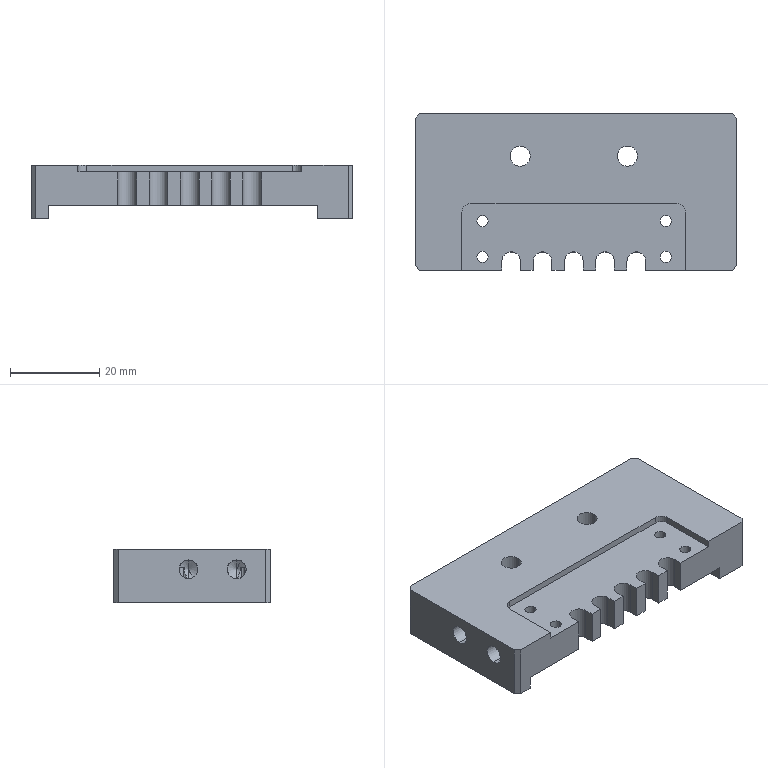Part | STEP file | 10000020471swp000-1 | 1 solid | 123 faces | box 72 x 35 x 12 mm | volume 19636 mm3 | cylinder 80 | plane 37 | cone 6 | commonest cylinder face diameters 1.5 x40 4.2 x22 2.5 x8 4.5 x4 8 x4 4 x2